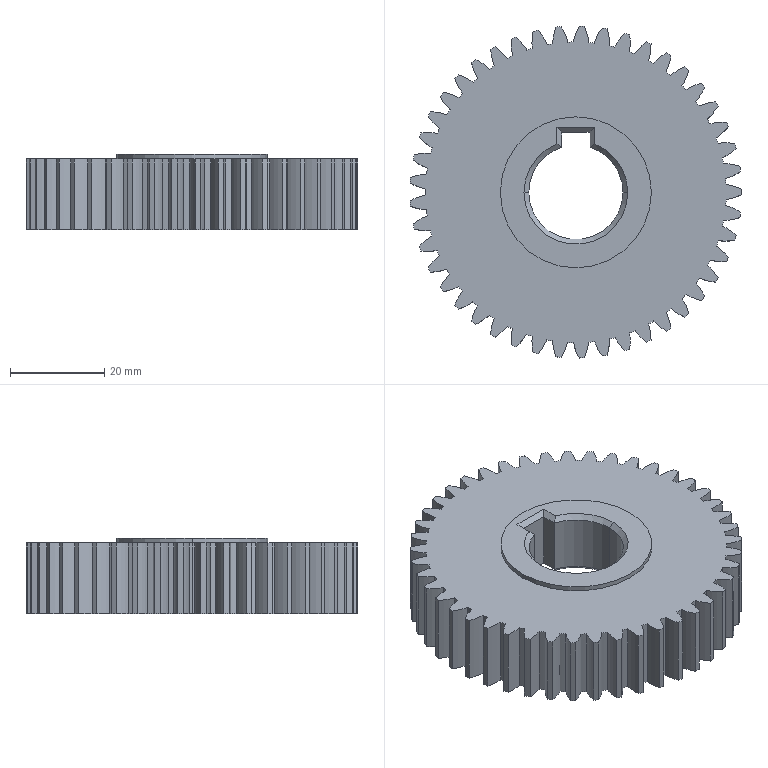Part | SolidWorks | features ICE 4, Chamfer 1, CirPattern 1, Extrusion 1 | 1 solid | 214 faces | box 70.282 x 70.32 x 16 mm | volume 46691 mm3 | cylinder 195 | plane 13 | cone 6 | commonest cylinder face diameters 23.086 x96 63.75 x46 70.5 x46 20 x3 32 x2 40 x2